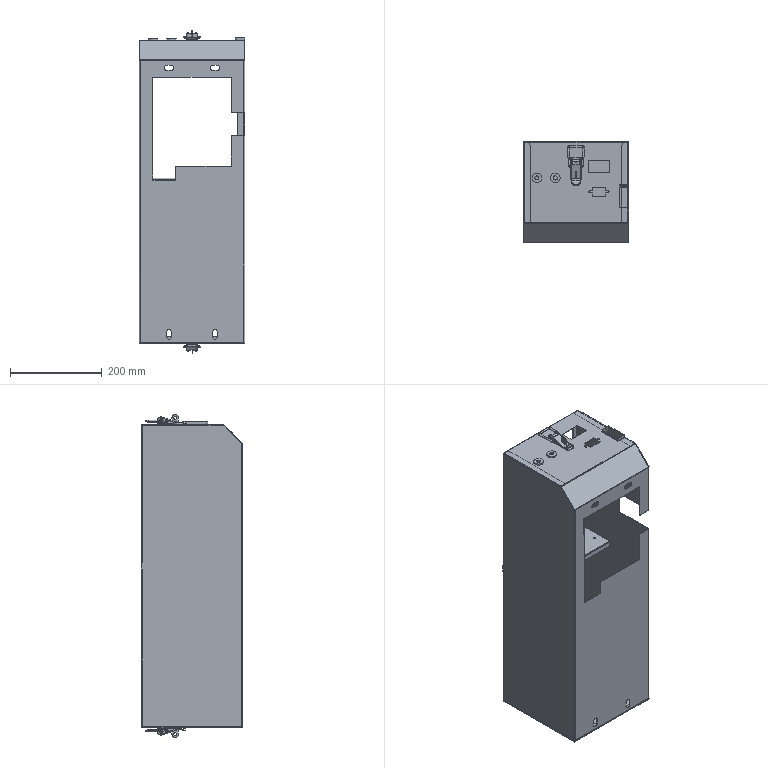Part | SolidWorks | 15 solids | 579 faces | box 230 x 220.134 x 702 mm | volume 564846 mm3 | plane 332 | cylinder 201 | spline 24 | torus 22 | commonest cylinder face diameters 4 x68 2 x32 5 x31 6 x12 14 x12 11 x10